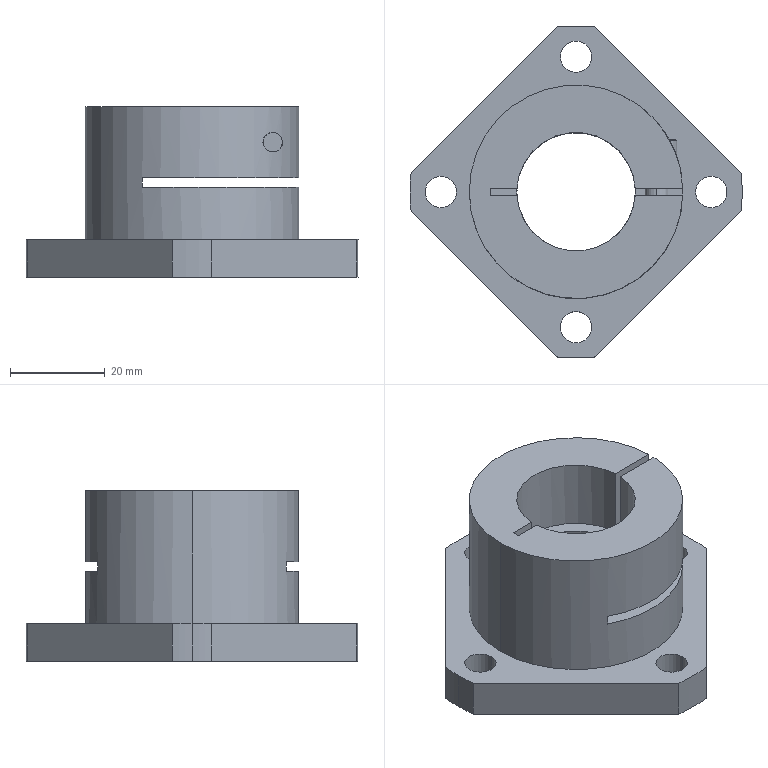Part | SolidWorks | features BaseBody 2 | 2 solids | 67 faces | box 70 x 70 x 36 mm | volume 47267 mm3 | plane 34 | cylinder 27 | cone 6 | commonest cylinder face diameters 6.6 x8 70 x5 4.134 x2 5 x2 5.6 x2 8.5 x2